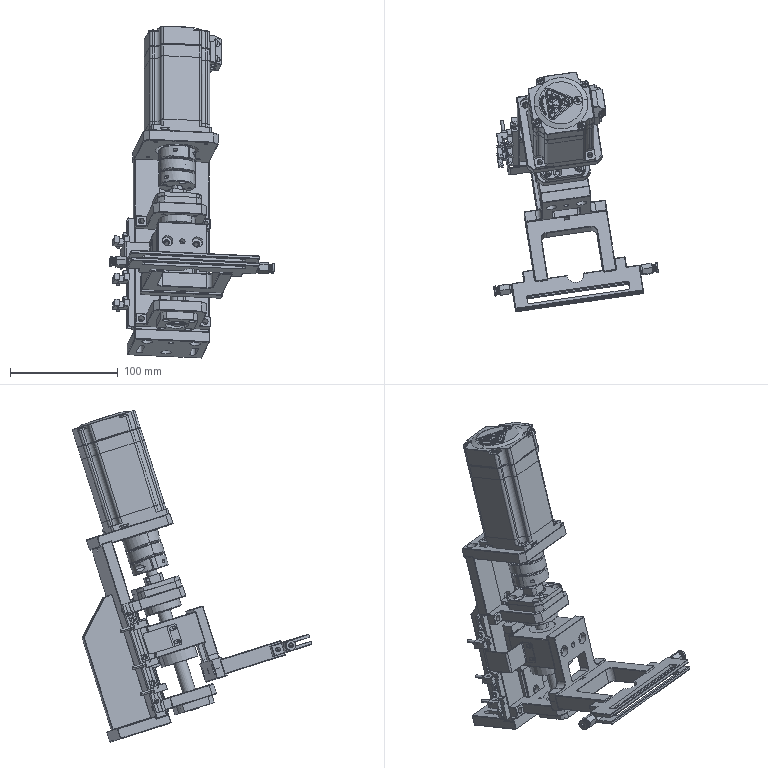Part | SolidWorks | features CompositeCurve 1 | 65 solids | 5238 faces | volume 638711 mm3 | plane 2535 | cylinder 1629 | spline 538 | cone 493 | torus 43 | commonest cylinder face diameters 3 x215 0.6 x116 2 x111 1 x98 3.3 x71 5.5 x66